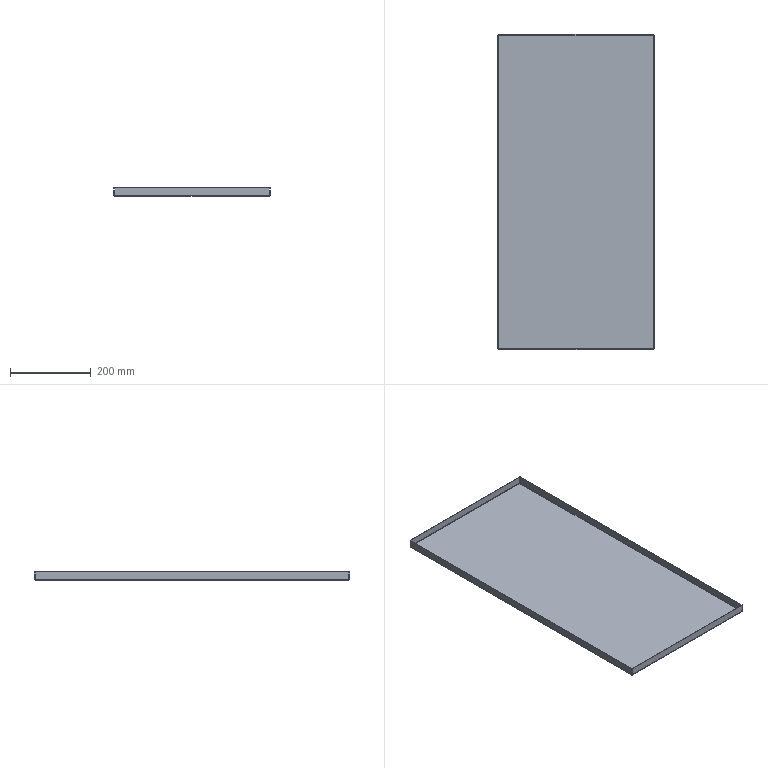Part | STEP file | X77-03010 | 1 solid | 38 faces | box 386 x 778 x 20 mm | volume 512333 mm3 | plane 22 | spline 8 | cylinder 8 | commonest cylinder face diameters 1.473 x4 4.473 x4